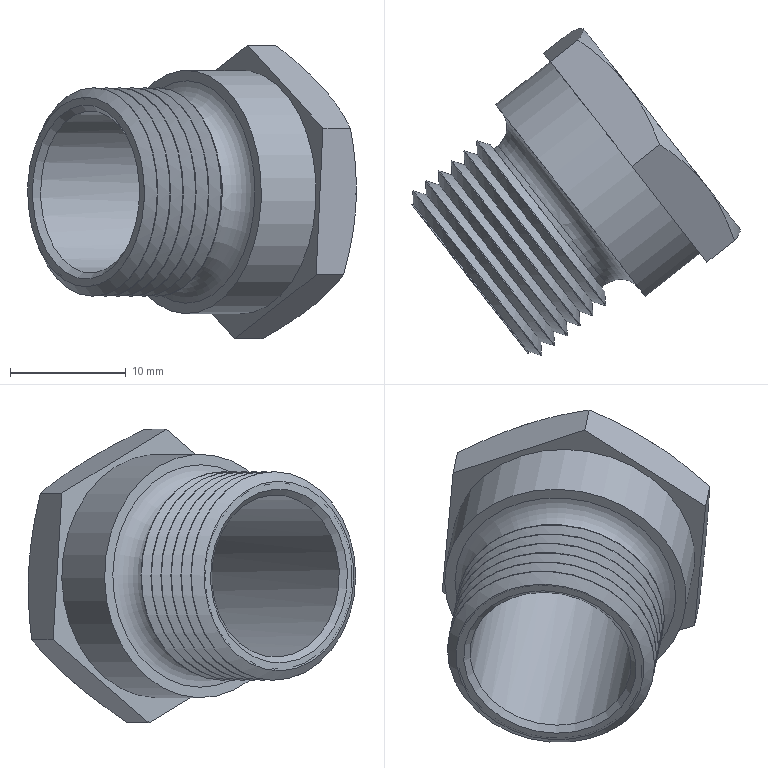Part | NX | features BREP 1 | 1 solid | 42 faces | box 28.365 x 28.243 x 25.334 mm | volume 2943 mm3 | cone 21 | plane 11 | cylinder 9 | torus 1 | commonest cylinder face diameters 18 x6 14 x1 15.2 x1 21 x1
STEP:
#1=CARTESIAN_POINT('',(-20.726,70.701,-110.314));
#2=VERTEX_POINT('',#1);
#3=CARTESIAN_POINT('',(-23.847,74.697,-117.75));
#4=DIRECTION('',(0.788,0.6157,0.));
#5=DIRECTION('',(0.3468,-0.4439,0.8262));
#6=AXIS2_PLACEMENT_3D('',#3,#4,#5);
#7=CIRCLE('',#6,9.);
#8=EDGE_CURVE('',#2,#2,#7,.T.);
#9=ORIENTED_EDGE('',*,*,#8,.T.);
#10=EDGE_LOOP('',(#9));
#11=FACE_BOUND('',#10,.T.);
#12=CARTESIAN_POINT('',(-26.925,78.726,-125.186));
#13=VERTEX_POINT('',#12);
#14=CARTESIAN_POINT('',(-23.803,74.731,-117.75));
#15=DIRECTION('',(-0.788,-0.6157,0.));
#16=DIRECTION('',(-0.3468,0.4439,-0.8262));
#17=AXIS2_PLACEMENT_3D('',#14,#15,#16);
#18=CIRCLE('',#17,9.);
#19=EDGE_CURVE('',#13,#13,#18,.T.);
#20=ORIENTED_EDGE('',*,*,#19,.T.);
#21=EDGE_LOOP('',(#20));
#22=FACE_BOUND('',#21,.T.);
#23=CARTESIAN_POINT('',(-25.559,73.359,-117.75));
#24=DIRECTION('',(0.788,0.6157,0.));
#25=DIRECTION('',(-0.3468,0.4439,-0.8262));
#26=AXIS2_PLACEMENT_3D('',#23,#24,#25);
#27=CYLINDRICAL_SURFACE('',#26,9.);
#28=ADVANCED_FACE('',(#11,#22),#27,.T.);
#29=CARTESIAN_POINT('',(-19.623,71.563,-110.314));
#30=VERTEX_POINT('',#29);
#31=CARTESIAN_POINT('',(-22.744,75.559,-117.75));
#32=DIRECTION('',(0.788,0.6157,0.));
#33=DIRECTION('',(0.3468,-0.4439,0.8262));
#34=AXIS2_PLACEMENT_3D('',#31,#32,#33);
#35=CIRCLE('',#34,9.);
#36=EDGE_CURVE('',#30,#30,#35,.T.);
#37=ORIENTED_EDGE('',*,*,#36,.T.);
#38=EDGE_LOOP('',(#37));
#39=FACE_BOUND('',#38,.T.);
#40=CARTESIAN_POINT('',(-25.822,79.588,-125.186));
#41=VERTEX_POINT('',#40);
#42=CARTESIAN_POINT('',(-22.7,75.593,-117.75));
#43=DIRECTION('',(-0.788,-0.6157,0.));
#44=DIRECTION('',(-0.3468,0.4439,-0.8262));
#45=AXIS2_PLACEMENT_3D('',#42,#43,#44);
#46=CIRCLE('',#45,9.);
#47=EDGE_CURVE('',#41,#41,#46,.T.);
#48=ORIENTED_EDGE('',*,*,#47,.T.);
#49=EDGE_LOOP('',(#48));
#50=FACE_BOUND('',#49,.T.);
#51=CARTESIAN_POINT('',(-25.559,73.359,-117.75));
#52=DIRECTION('',(0.788,0.6157,0.));
#53=DIRECTION('',(-0.3468,0.4439,-0.8262));
#54=AXIS2_PLACEMENT_3D('',#51,#52,#53);
#55=CYLINDRICAL_SURFACE('',#54,9.);
#56=ADVANCED_FACE('',(#39,#50),#55,.T.);
#57=CARTESIAN_POINT('',(-18.52,72.425,-110.314));
#58=VERTEX_POINT('',#57);
#59=CARTESIAN_POINT('',(-21.641,76.42,-117.75));
#60=DIRECTION('',(0.788,0.6157,0.));
#61=DIRECTION('',(0.3468,-0.4439,0.8262));
#62=AXIS2_PLACEMENT_3D('',#59,#60,#61);
#63=CIRCLE('',#62,9.);
#64=EDGE_CURVE('',#58,#58,#63,.T.);
#65=ORIENTED_EDGE('',*,*,#64,.T.);
#66=EDGE_LOOP('',(#65));
#67=FACE_BOUND('',#66,.T.);
#68=CARTESIAN_POINT('',(-24.718,80.45,-125.186));
#69=VERTEX_POINT('',#68);
#70=CARTESIAN_POINT('',(-21.597,76.455,-117.75));
#71=DIRECTION('',(-0.788,-0.6157,0.));
#72=DIRECTION('',(-0.3468,0.4439,-0.8262));
#73=AXIS2_PLACEMENT_3D('',#70,#71,#72);
#74=CIRCLE('',#73,9.);
#75=EDGE_CURVE('',#69,#69,#74,.T.);
#76=ORIENTED_EDGE('',*,*,#75,.T.);
#77=EDGE_LOOP('',(#76));
#78=FACE_BOUND('',#77,.T.);
#79=CARTESIAN_POINT('',(-25.559,73.359,-117.75));
#80=DIRECTION('',(0.788,0.6157,0.));
#81=DIRECTION('',(-0.3468,0.4439,-0.8262));
#82=AXIS2_PLACEMENT_3D('',#79,#80,#81);
#83=CYLINDRICAL_SURFACE('',#82,9.);
#84=ADVANCED_FACE('',(#67,#78),#83,.T.);
#85=CARTESIAN_POINT('',(-17.416,73.287,-110.314));
#86=VERTEX_POINT('',#85);
#87=CARTESIAN_POINT('',(-20.538,77.282,-117.75));
#88=DIRECTION('',(0.788,0.6157,0.));
#89=DIRECTION('',(0.3468,-0.4439,0.8262));
#90=AXIS2_PLACEMENT_3D('',#87,#88,#89);
#91=CIRCLE('',#90,9.);
#92=EDGE_CURVE('',#86,#86,#91,.T.);
#93=ORIENTED_EDGE('',*,*,#92,.T.);
#94=EDGE_LOOP('',(#93));
#95=FACE_BOUND('',#94,.T.);
#96=CARTESIAN_POINT('',(-23.615,81.312,-125.186));
#97=VERTEX_POINT('',#96);
#98=CARTESIAN_POINT('',(-20.494,77.317,-117.75));
#99=DIRECTION('',(-0.788,-0.6157,0.));
#100=DIRECTION('',(-0.3468,0.4439,-0.8262));
#101=AXIS2_PLACEMENT_3D('',#98,#99,#100);
#102=CIRCLE('',#101,9.);
#103=EDGE_CURVE('',#97,#97,#102,.T.);
#104=ORIENTED_EDGE('',*,*,#103,.T.);
#105=EDGE_LOOP('',(#104));
#106=FACE_BOUND('',#105,.T.);
#107=CARTESIAN_POINT('',(-25.559,73.359,-117.75));
#108=DIRECTION('',(0.788,0.6157,0.));
#109=DIRECTION('',(-0.3468,0.4439,-0.8262));
#110=AXIS2_PLACEMENT_3D('',#107,#108,#109);
#111=CYLINDRICAL_SURFACE('',#110,9.);
#112=ADVANCED_FACE('',(#95,#106),#111,.T.);
#113=CARTESIAN_POINT('',(-16.313,74.149,-110.314));
#114=VERTEX_POINT('',#113);
#115=CARTESIAN_POINT('',(-19.435,78.144,-117.75));
#116=DIRECTION('',(0.788,0.6157,0.));
#117=DIRECTION('',(0.3468,-0.4439,0.8262));
#118=AXIS2_PLACEMENT_3D('',#115,#116,#117);
#119=CIRCLE('',#118,9.);
#120=EDGE_CURVE('',#114,#114,#119,.T.);
#121=ORIENTED_EDGE('',*,*,#120,.T.);
#122=EDGE_LOOP('',(#121));
#123=FACE_BOUND('',#122,.T.);
#124=CARTESIAN_POINT('',(-22.512,82.174,-125.186));
#125=VERTEX_POINT('',#124);
#126=CARTESIAN_POINT('',(-19.391,78.179,-117.75));
#127=DIRECTION('',(-0.788,-0.6157,0.));
#128=DIRECTION('',(-0.3468,0.4439,-0.8262));
#129=AXIS2_PLACEMENT_3D('',#126,#127,#128);
#130=CIRCLE('',#129,9.);
#131=EDGE_CURVE('',#125,#125,#130,.T.);
#132=ORIENTED_EDGE('',*,*,#131,.T.);
#133=EDGE_LOOP('',(#132));
#134=FACE_BOUND('',#133,.T.);
#135=CARTESIAN_POINT('',(-25.559,73.359,-117.75));
#136=DIRECTION('',(0.788,0.6157,0.));
#137=DIRECTION('',(-0.3468,0.4439,-0.8262));
#138=AXIS2_PLACEMENT_3D('',#135,#136,#137);
#139=CYLINDRICAL_SURFACE('',#138,9.);
#140=ADVANCED_FACE('',(#123,#134),#139,.T.);
#141=CARTESIAN_POINT('',(-3.324,77.415,-124.905));
#142=VERTEX_POINT('',#141);
#143=CARTESIAN_POINT('',(-6.071,82.526,-127.66));
#144=VERTEX_POINT('',#143);
#145=CARTESIAN_POINT('',(-3.324,77.415,-124.905));
#146=CARTESIAN_POINT('',(-4.003,79.256,-125.805));
#147=CARTESIAN_POINT('',(-4.87,80.988,-126.719));
#148=CARTESIAN_POINT('',(-6.071,82.526,-127.66));
#149=B_SPLINE_CURVE_WITH_KNOTS('',3,(#145,#146,#147,#148),.UNSPECIFIED.,.F.,.F.,(4,4),(0.,0.006423),.UNSPECIFIED.);
#150=EDGE_CURVE('',#142,#144,#149,.T.);
#151=ORIENTED_EDGE('',*,*,#150,.F.);
#152=CARTESIAN_POINT('',(-5.703,75.557,-124.905));
#153=VERTEX_POINT('',#152);
#154=CARTESIAN_POINT('',(-5.703,75.557,-124.905));
#155=DIRECTION('',(0.788,0.6157,0.));
#156=VECTOR('',#155,1000.);
#157=LINE('',#154,#156);
#158=EDGE_CURVE('',#153,#142,#157,.T.);
#159=ORIENTED_EDGE('',*,*,#158,.F.);
#160=CARTESIAN_POINT('',(-12.747,84.573,-130.417));
#161=VERTEX_POINT('',#160);
#162=CARTESIAN_POINT('',(-12.747,84.573,-130.417));
#163=DIRECTION('',(0.5546,-0.7099,0.4341));
#164=VECTOR('',#163,1000.);
#165=LINE('',#162,#164);
#166=EDGE_CURVE('',#161,#153,#165,.T.);
#167=ORIENTED_EDGE('',*,*,#166,.F.);
#168=CARTESIAN_POINT('',(-10.369,86.43,-130.417));
#169=VERTEX_POINT('',#168);
#170=CARTESIAN_POINT('',(-12.747,84.573,-130.417));
#171=DIRECTION('',(0.788,0.6157,0.));
#172=VECTOR('',#171,1000.);
#173=LINE('',#170,#172);
#174=EDGE_CURVE('',#161,#169,#173,.T.);
#175=ORIENTED_EDGE('',*,*,#174,.T.);
#176=CARTESIAN_POINT('',(-6.071,82.526,-127.66));
#177=CARTESIAN_POINT('',(-7.274,84.065,-128.601));
#178=CARTESIAN_POINT('',(-8.746,85.326,-129.516));
#179=CARTESIAN_POINT('',(-10.369,86.43,-130.417));
#180=B_SPLINE_CURVE_WITH_KNOTS('',3,(#176,#177,#178,#179),.UNSPECIFIED.,.F.,.F.,(4,4),(0.,0.006428),.UNSPECIFIED.);
#181=EDGE_CURVE('',#144,#169,#180,.T.);
#182=ORIENTED_EDGE('',*,*,#181,.F.);
#183=EDGE_LOOP('',(#151,#159,#167,#175,#182));
#184=FACE_BOUND('',#183,.T.);
#185=CARTESIAN_POINT('',(-12.747,84.573,-130.417));
#186=DIRECTION('',(-0.2672,0.342,0.9009));
#187=DIRECTION('',(0.5546,-0.7099,0.4341));
#188=AXIS2_PLACEMENT_3D('',#185,#186,#187);
#189=PLANE('',#188);
#190=ADVANCED_FACE('',(#184),#189,.F.);
#191=CARTESIAN_POINT('',(-2.739,76.664,-112.24));
#192=VERTEX_POINT('',#191);
#193=CARTESIAN_POINT('',(-2.258,77.645,-118.575));
#194=VERTEX_POINT('',#193);
#195=CARTESIAN_POINT('',(-2.739,76.664,-112.24));
#196=CARTESIAN_POINT('',(-2.362,77.156,-114.31));
#197=CARTESIAN_POINT('',(-2.157,77.516,-116.413));
#198=CARTESIAN_POINT('',(-2.258,77.645,-118.575));
#199=B_SPLINE_CURVE_WITH_KNOTS('',3,(#195,#196,#197,#198),.UNSPECIFIED.,.F.,.F.,(4,4),(0.,0.006428),.UNSPECIFIED.);
#200=EDGE_CURVE('',#192,#194,#199,.T.);
#201=ORIENTED_EDGE('',*,*,#200,.F.);
#202=CARTESIAN_POINT('',(-5.116,74.806,-112.24));
#203=VERTEX_POINT('',#202);
#204=CARTESIAN_POINT('',(-5.116,74.806,-112.24));
#205=DIRECTION('',(0.788,0.6157,0.));
#206=VECTOR('',#205,1000.);
#207=LINE('',#204,#206);
#208=EDGE_CURVE('',#203,#192,#207,.T.);
#209=ORIENTED_EDGE('',*,*,#208,.F.);
#210=CARTESIAN_POINT('',(-5.116,74.806,-112.24));
#211=DIRECTION('',(0.04618,-0.05911,0.9972));
#212=VECTOR('',#211,1000.);
#213=LINE('',#210,#212);
#214=EDGE_CURVE('',#153,#203,#213,.T.);
#215=ORIENTED_EDGE('',*,*,#214,.F.);
#216=ORIENTED_EDGE('',*,*,#158,.T.);
#217=CARTESIAN_POINT('',(-2.258,77.645,-118.575));
#218=CARTESIAN_POINT('',(-2.358,77.773,-120.735));
#219=CARTESIAN_POINT('',(-2.757,77.661,-122.837));
#220=CARTESIAN_POINT('',(-3.324,77.415,-124.905));
#221=B_SPLINE_CURVE_WITH_KNOTS('',3,(#217,#218,#219,#220),.UNSPECIFIED.,.F.,.F.,(4,4),(0.,0.006423),.UNSPECIFIED.);
#222=EDGE_CURVE('',#194,#142,#221,.T.);
#223=ORIENTED_EDGE('',*,*,#222,.F.);
#224=EDGE_LOOP('',(#201,#209,#215,#216,#223));
#225=FACE_BOUND('',#224,.T.);
#226=CARTESIAN_POINT('',(-5.116,74.806,-112.24));
#227=DIRECTION('',(-0.6139,0.7858,0.07501));
#228=DIRECTION('',(0.04618,-0.05911,0.9972));
#229=AXIS2_PLACEMENT_3D('',#226,#227,#228);
#230=PLANE('',#229);
#231=ADVANCED_FACE('',(#225),#230,.F.);
#232=CARTESIAN_POINT('',(-9.202,84.936,-105.083));
#233=VERTEX_POINT('',#232);
#234=CARTESIAN_POINT('',(-5.196,81.405,-108.662));
#235=VERTEX_POINT('',#234);
#236=CARTESIAN_POINT('',(-9.202,84.936,-105.083));
#237=CARTESIAN_POINT('',(-7.674,83.953,-106.252));
#238=CARTESIAN_POINT('',(-6.299,82.817,-107.44));
#239=CARTESIAN_POINT('',(-5.196,81.405,-108.662));
#240=B_SPLINE_CURVE_WITH_KNOTS('',3,(#236,#237,#238,#239),.UNSPECIFIED.,.F.,.F.,(4,4),(0.,0.006428),.UNSPECIFIED.);
#241=EDGE_CURVE('',#233,#235,#240,.T.);
#242=ORIENTED_EDGE('',*,*,#241,.F.);
#243=CARTESIAN_POINT('',(-11.579,83.078,-105.083));
#244=VERTEX_POINT('',#243);
#245=CARTESIAN_POINT('',(-11.579,83.078,-105.083));
#246=DIRECTION('',(0.788,0.6157,0.));
#247=VECTOR('',#246,1000.);
#248=LINE('',#245,#247);
#249=EDGE_CURVE('',#244,#233,#248,.T.);
#250=ORIENTED_EDGE('',*,*,#249,.F.);
#251=CARTESIAN_POINT('',(-11.579,83.078,-105.083));
#252=DIRECTION('',(-0.5087,0.6511,0.5634));
#253=VECTOR('',#252,1000.);
#254=LINE('',#251,#253);
#255=EDGE_CURVE('',#203,#244,#254,.T.);
#256=ORIENTED_EDGE('',*,*,#255,.F.);
#257=ORIENTED_EDGE('',*,*,#208,.T.);
#258=CARTESIAN_POINT('',(-5.196,81.405,-108.662));
#259=CARTESIAN_POINT('',(-4.093,79.993,-109.883));
#260=CARTESIAN_POINT('',(-3.322,78.384,-111.071));
#261=CARTESIAN_POINT('',(-2.739,76.664,-112.24));
#262=B_SPLINE_CURVE_WITH_KNOTS('',3,(#258,#259,#260,#261),.UNSPECIFIED.,.F.,.F.,(4,4),(0.,0.006428),.UNSPECIFIED.);
#263=EDGE_CURVE('',#235,#192,#262,.T.);
#264=ORIENTED_EDGE('',*,*,#263,.F.);
#265=EDGE_LOOP('',(#242,#250,#256,#257,#264));
#266=FACE_BOUND('',#265,.T.);
#267=CARTESIAN_POINT('',(-11.579,83.078,-105.083));
#268=DIRECTION('',(-0.3468,0.4439,-0.8262));
#269=DIRECTION('',(-0.788,-0.6157,0.));
#270=AXIS2_PLACEMENT_3D('',#267,#268,#269);
#271=PLANE('',#270);
#272=ADVANCED_FACE('',(#266),#271,.F.);
#273=CARTESIAN_POINT('',(-16.244,93.953,-110.595));
#274=VERTEX_POINT('',#273);
#275=CARTESIAN_POINT('',(-11.95,90.051,-107.84));
#276=VERTEX_POINT('',#275);
#277=CARTESIAN_POINT('',(-16.244,93.953,-110.595));
#278=CARTESIAN_POINT('',(-14.623,92.849,-109.695));
#279=CARTESIAN_POINT('',(-13.152,91.589,-108.781));
#280=CARTESIAN_POINT('',(-11.95,90.051,-107.84));
#281=B_SPLINE_CURVE_WITH_KNOTS('',3,(#277,#278,#279,#280),.UNSPECIFIED.,.F.,.F.,(4,4),(0.,0.006423),.UNSPECIFIED.);
#282=EDGE_CURVE('',#274,#276,#281,.T.);
#283=ORIENTED_EDGE('',*,*,#282,.F.);
#284=CARTESIAN_POINT('',(-18.623,92.094,-110.595));
#285=VERTEX_POINT('',#284);
#286=CARTESIAN_POINT('',(-18.623,92.094,-110.595));
#287=DIRECTION('',(0.788,0.6157,0.));
#288=VECTOR('',#287,1000.);
#289=LINE('',#286,#288);
#290=EDGE_CURVE('',#285,#274,#289,.T.);
#291=ORIENTED_EDGE('',*,*,#290,.F.);
#292=CARTESIAN_POINT('',(-11.579,83.078,-105.083));
#293=DIRECTION('',(-0.5546,0.7099,-0.4341));
#294=VECTOR('',#293,1000.);
#295=LINE('',#292,#294);
#296=EDGE_CURVE('',#244,#285,#295,.T.);
#297=ORIENTED_EDGE('',*,*,#296,.F.);
#298=ORIENTED_EDGE('',*,*,#249,.T.);
#299=CARTESIAN_POINT('',(-11.95,90.051,-107.84));
#300=CARTESIAN_POINT('',(-10.748,88.511,-106.899));
#301=CARTESIAN_POINT('',(-9.88,86.778,-105.984));
#302=CARTESIAN_POINT('',(-9.202,84.936,-105.083));
#303=B_SPLINE_CURVE_WITH_KNOTS('',3,(#299,#300,#301,#302),.UNSPECIFIED.,.F.,.F.,(4,4),(0.,0.006428),.UNSPECIFIED.);
#304=EDGE_CURVE('',#276,#233,#303,.T.);
#305=ORIENTED_EDGE('',*,*,#304,.F.);
#306=EDGE_LOOP('',(#283,#291,#297,#298,#305));
#307=FACE_BOUND('',#306,.T.);
#308=CARTESIAN_POINT('',(-11.579,83.078,-105.083));
#309=DIRECTION('',(0.2672,-0.342,-0.9009));
#310=DIRECTION('',(-0.5546,0.7099,-0.4341));
#311=AXIS2_PLACEMENT_3D('',#308,#309,#310);
#312=PLANE('',#311);
#313=ADVANCED_FACE('',(#307),#312,.F.);
#314=CARTESIAN_POINT('',(-16.832,94.702,-123.26));
#315=VERTEX_POINT('',#314);
#316=CARTESIAN_POINT('',(-15.764,94.932,-116.925));
#317=VERTEX_POINT('',#316);
#318=CARTESIAN_POINT('',(-16.832,94.702,-123.26));
#319=CARTESIAN_POINT('',(-16.264,94.949,-121.19));
#320=CARTESIAN_POINT('',(-15.864,95.06,-119.087));
#321=CARTESIAN_POINT('',(-15.764,94.932,-116.925));
#322=B_SPLINE_CURVE_WITH_KNOTS('',3,(#318,#319,#320,#321),.UNSPECIFIED.,.F.,.F.,(4,4),(0.,0.006428),.UNSPECIFIED.);
#323=EDGE_CURVE('',#315,#317,#322,.T.);
#324=ORIENTED_EDGE('',*,*,#323,.F.);
#325=CARTESIAN_POINT('',(-19.209,92.845,-123.26));
#326=VERTEX_POINT('',#325);
#327=CARTESIAN_POINT('',(-19.209,92.845,-123.26));
#328=DIRECTION('',(0.788,0.6157,0.));
#329=VECTOR('',#328,1000.);
#330=LINE('',#327,#329);
#331=EDGE_CURVE('',#326,#315,#330,.T.);
#332=ORIENTED_EDGE('',*,*,#331,.F.);
#333=CARTESIAN_POINT('',(-19.209,92.845,-123.26));
#334=DIRECTION('',(-0.04618,0.05911,-0.9972));
#335=VECTOR('',#334,1000.);
#336=LINE('',#333,#335);
#337=EDGE_CURVE('',#285,#326,#336,.T.);
#338=ORIENTED_EDGE('',*,*,#337,.F.);
#339=ORIENTED_EDGE('',*,*,#290,.T.);
#340=CARTESIAN_POINT('',(-15.764,94.932,-116.925));
#341=CARTESIAN_POINT('',(-15.664,94.804,-114.765));
#342=CARTESIAN_POINT('',(-15.869,94.444,-112.663));
#343=CARTESIAN_POINT('',(-16.244,93.953,-110.595));
#344=B_SPLINE_CURVE_WITH_KNOTS('',3,(#340,#341,#342,#343),.UNSPECIFIED.,.F.,.F.,(4,4),(0.,0.006423),.UNSPECIFIED.);
#345=EDGE_CURVE('',#317,#274,#344,.T.);
#346=ORIENTED_EDGE('',*,*,#345,.F.);
#347=EDGE_LOOP('',(#324,#332,#338,#339,#346));
#348=FACE_BOUND('',#347,.T.);
#349=CARTESIAN_POINT('',(-19.209,92.845,-123.26));
#350=DIRECTION('',(0.6139,-0.7858,-0.07501));
#351=DIRECTION('',(-0.04618,0.05911,-0.9972));
#352=AXIS2_PLACEMENT_3D('',#349,#350,#351);
#353=PLANE('',#352);
#354=ADVANCED_FACE('',(#348),#353,.F.);
#355=CARTESIAN_POINT('',(-12.826,91.172,-126.838));
#356=VERTEX_POINT('',#355);
#357=CARTESIAN_POINT('',(-10.369,86.43,-130.417));
#358=CARTESIAN_POINT('',(-10.953,88.151,-129.248));
#359=CARTESIAN_POINT('',(-11.723,89.76,-128.06));
#360=CARTESIAN_POINT('',(-12.826,91.172,-126.838));
#361=B_SPLINE_CURVE_WITH_KNOTS('',3,(#357,#358,#359,#360),.UNSPECIFIED.,.F.,.F.,(4,4),(0.,0.006428),.UNSPECIFIED.);
#362=EDGE_CURVE('',#169,#356,#361,.T.);
#363=ORIENTED_EDGE('',*,*,#362,.F.);
#364=ORIENTED_EDGE('',*,*,#174,.F.);
#365=CARTESIAN_POINT('',(-19.209,92.845,-123.26));
#366=DIRECTION('',(0.5087,-0.6511,-0.5634));
#367=VECTOR('',#366,1000.);
#368=LINE('',#365,#367);
#369=EDGE_CURVE('',#326,#161,#368,.T.);
#370=ORIENTED_EDGE('',*,*,#369,.F.);
#371=ORIENTED_EDGE('',*,*,#331,.T.);
#372=CARTESIAN_POINT('',(-12.826,91.172,-126.838));
#373=CARTESIAN_POINT('',(-13.929,92.583,-125.617));
#374=CARTESIAN_POINT('',(-15.304,93.72,-124.429));
#375=CARTESIAN_POINT('',(-16.832,94.702,-123.26));
#376=B_SPLINE_CURVE_WITH_KNOTS('',3,(#372,#373,#374,#375),.UNSPECIFIED.,.F.,.F.,(4,4),(0.,0.006428),.UNSPECIFIED.);
#377=EDGE_CURVE('',#356,#315,#376,.T.);
#378=ORIENTED_EDGE('',*,*,#377,.F.);
#379=EDGE_LOOP('',(#363,#364,#370,#371,#378));
#380=FACE_BOUND('',#379,.T.);
#381=CARTESIAN_POINT('',(-19.209,92.845,-123.26));
#382=DIRECTION('',(0.3468,-0.4439,0.8262));
#383=DIRECTION('',(0.788,0.6157,0.));
#384=AXIS2_PLACEMENT_3D('',#381,#382,#383);
#385=PLANE('',#384);
#386=ADVANCED_FACE('',(#380),#385,.F.);
#387=ORIENTED_EDGE('',*,*,#166,.T.);
#388=ORIENTED_EDGE('',*,*,#214,.T.);
#389=ORIENTED_EDGE('',*,*,#255,.T.);
#390=ORIENTED_EDGE('',*,*,#296,.T.);
#391=ORIENTED_EDGE('',*,*,#337,.T.);
#392=ORIENTED_EDGE('',*,*,#369,.T.);
#393=EDGE_LOOP('',(#387,#388,#389,#390,#391,#392));
#394=FACE_BOUND('',#393,.T.);
#395=CARTESIAN_POINT('',(-15.805,88.487,-126.425));
#396=VERTEX_POINT('',#395);
#397=CARTESIAN_POINT('',(-12.163,83.826,-117.75));
#398=DIRECTION('',(-0.788,-0.6157,0.));
#399=DIRECTION('',(-0.3468,0.4439,-0.8262));
#400=AXIS2_PLACEMENT_3D('',#397,#398,#399);
#401=CIRCLE('',#400,10.5);
#402=EDGE_CURVE('',#396,#396,#401,.T.);
#403=ORIENTED_EDGE('',*,*,#402,.F.);
#404=EDGE_LOOP('',(#403));
#405=FACE_BOUND('',#404,.T.);
#406=CARTESIAN_POINT('',(1.341,66.541,-119.392));
#407=DIRECTION('',(0.788,0.6157,0.));
#408=DIRECTION('',(-0.3468,0.4439,-0.8262));
#409=AXIS2_PLACEMENT_3D('',#406,#407,#408);
#410=PLANE('',#409);
#411=ADVANCED_FACE('',(#394,#405),#410,.F.);
#412=CARTESIAN_POINT('',(-20.533,84.793,-126.425));
#413=VERTEX_POINT('',#412);
#414=CARTESIAN_POINT('',(-16.891,80.132,-117.75));
#415=DIRECTION('',(-0.788,-0.6157,0.));
#416=DIRECTION('',(-0.3468,0.4439,-0.8262));
#417=AXIS2_PLACEMENT_3D('',#414,#415,#416);
#418=CIRCLE('',#417,10.5);
#419=EDGE_CURVE('',#413,#413,#418,.T.);
#420=ORIENTED_EDGE('',*,*,#419,.F.);
#421=EDGE_LOOP('',(#420));
#422=FACE_BOUND('',#421,.T.);
#423=ORIENTED_EDGE('',*,*,#402,.T.);
#424=EDGE_LOOP('',(#423));
#425=FACE_BOUND('',#424,.T.);
#426=CARTESIAN_POINT('',(-16.891,80.132,-117.75));
#427=DIRECTION('',(0.788,0.6157,0.));
#428=DIRECTION('',(-0.3468,0.4439,-0.8262));
#429=AXIS2_PLACEMENT_3D('',#426,#427,#428);
#430=CYLINDRICAL_SURFACE('',#429,10.5);
#431=ADVANCED_FACE('',(#422,#425),#430,.T.);
#432=CARTESIAN_POINT('',(-20.221,84.393,-125.682));
#433=VERTEX_POINT('',#432);
#434=CARTESIAN_POINT('',(-16.891,80.132,-117.75));
#435=DIRECTION('',(0.788,0.6157,0.));
#436=DIRECTION('',(-0.3468,0.4439,-0.8262));
#437=AXIS2_PLACEMENT_3D('',#434,#435,#436);
#438=CIRCLE('',#437,9.6);
#439=EDGE_CURVE('',#433,#433,#438,.T.);
#440=ORIENTED_EDGE('',*,*,#439,.T.);
#441=EDGE_LOOP('',(#440));
#442=FACE_BOUND('',#441,.T.);
#443=ORIENTED_EDGE('',*,*,#419,.T.);
#444=EDGE_LOOP('',(#443));
#445=FACE_BOUND('',#444,.T.);
#446=CARTESIAN_POINT('',(-16.891,80.132,-117.75));
#447=DIRECTION('',(-0.788,-0.6157,0.));
#448=DIRECTION('',(0.3468,-0.4439,0.8262));
#449=AXIS2_PLACEMENT_3D('',#446,#447,#448);
#450=PLANE('',#449);
#451=ADVANCED_FACE('',(#442,#445),#450,.T.);
#452=ORIENTED_EDGE('',*,*,#263,.T.);
#453=ORIENTED_EDGE('',*,*,#200,.T.);
#454=CARTESIAN_POINT('',(-9.011,86.288,-117.75));
#455=DIRECTION('',(0.788,0.6157,0.));
#456=DIRECTION('',(0.3468,-0.4439,0.8262));
#457=AXIS2_PLACEMENT_3D('',#454,#455,#456);
#458=CIRCLE('',#457,11.);
#459=EDGE_CURVE('',#235,#194,#458,.T.);
#460=ORIENTED_EDGE('',*,*,#459,.F.);
#461=EDGE_LOOP('',(#452,#453,#460));
#462=FACE_BOUND('',#461,.T.);
#463=CARTESIAN_POINT('',(-9.011,86.288,-117.75));
#464=DIRECTION('',(-0.788,-0.6157,0.));
#465=DIRECTION('',(-0.3468,0.4439,-0.8262));
#466=AXIS2_PLACEMENT_3D('',#463,#464,#465);
#467=CONICAL_SURFACE('',#466,11.,1.047);
#468=ADVANCED_FACE('',(#462),#467,.T.);
#469=ORIENTED_EDGE('',*,*,#222,.T.);
#470=ORIENTED_EDGE('',*,*,#150,.T.);
#471=CARTESIAN_POINT('',(-9.011,86.288,-117.75));
#472=DIRECTION('',(-0.788,-0.6157,0.));
#473=DIRECTION('',(0.3468,-0.4439,0.8262));
#474=AXIS2_PLACEMENT_3D('',#471,#472,#473);
#475=CIRCLE('',#474,11.);
#476=EDGE_CURVE('',#144,#194,#475,.T.);
#477=ORIENTED_EDGE('',*,*,#476,.T.);
#478=EDGE_LOOP('',(#469,#470,#477));
#479=FACE_BOUND('',#478,.T.);
#480=CARTESIAN_POINT('',(-9.011,86.288,-117.75));
#481=DIRECTION('',(-0.788,-0.6157,0.));
#482=DIRECTION('',(-0.3468,0.4439,-0.8262));
#483=AXIS2_PLACEMENT_3D('',#480,#481,#482);
#484=CONICAL_SURFACE('',#483,11.,1.047);
#485=ADVANCED_FACE('',(#479),#484,.T.);
#486=ORIENTED_EDGE('',*,*,#181,.T.);
#487=ORIENTED_EDGE('',*,*,#362,.T.);
#488=CARTESIAN_POINT('',(-9.011,86.288,-117.75));
#489=DIRECTION('',(-0.788,-0.6157,0.));
#490=DIRECTION('',(0.3468,-0.4439,0.8262));
#491=AXIS2_PLACEMENT_3D('',#488,#489,#490);
#492=CIRCLE('',#491,11.);
#493=EDGE_CURVE('',#356,#144,#492,.T.);
#494=ORIENTED_EDGE('',*,*,#493,.T.);
#495=EDGE_LOOP('',(#486,#487,#494));
#496=FACE_BOUND('',#495,.T.);
#497=CARTESIAN_POINT('',(-9.011,86.288,-117.75));
#498=DIRECTION('',(-0.788,-0.6157,0.));
#499=DIRECTION('',(-0.3468,0.4439,-0.8262));
#500=AXIS2_PLACEMENT_3D('',#497,#498,#499);
#501=CONICAL_SURFACE('',#500,11.,1.047);
#502=ADVANCED_FACE('',(#496),#501,.T.);
#503=ORIENTED_EDGE('',*,*,#323,.T.);
#504=CARTESIAN_POINT('',(-9.011,86.288,-117.75));
#505=DIRECTION('',(-0.788,-0.6157,0.));
#506=DIRECTION('',(0.3468,-0.4439,0.8262));
#507=AXIS2_PLACEMENT_3D('',#504,#505,#506);
#508=CIRCLE('',#507,11.);
#509=EDGE_CURVE('',#317,#356,#508,.T.);
#510=ORIENTED_EDGE('',*,*,#509,.T.);
#511=ORIENTED_EDGE('',*,*,#377,.T.);
#512=EDGE_LOOP('',(#503,#510,#511));
#513=FACE_BOUND('',#512,.T.);
#514=CARTESIAN_POINT('',(-9.011,86.288,-117.75));
#515=DIRECTION('',(-0.788,-0.6157,0.));
#516=DIRECTION('',(-0.3468,0.4439,-0.8262));
#517=AXIS2_PLACEMENT_3D('',#514,#515,#516);
#518=CONICAL_SURFACE('',#517,11.,1.047);
#519=ADVANCED_FACE('',(#513),#518,.T.);
#520=ORIENTED_EDGE('',*,*,#282,.T.);
#521=CARTESIAN_POINT('',(-9.011,86.288,-117.75));
#522=DIRECTION('',(-0.788,-0.6157,0.));
#523=DIRECTION('',(0.3468,-0.4439,0.8262));
#524=AXIS2_PLACEMENT_3D('',#521,#522,#523);
#525=CIRCLE('',#524,11.);
#526=EDGE_CURVE('',#276,#317,#525,.T.);
#527=ORIENTED_EDGE('',*,*,#526,.T.);
#528=ORIENTED_EDGE('',*,*,#345,.T.);
#529=EDGE_LOOP('',(#520,#527,#528));
#530=FACE_BOUND('',#529,.T.);
#531=CARTESIAN_POINT('',(-9.011,86.288,-117.75));
#532=DIRECTION('',(-0.788,-0.6157,0.));
#533=DIRECTION('',(-0.3468,0.4439,-0.8262));
#534=AXIS2_PLACEMENT_3D('',#531,#532,#533);
#535=CONICAL_SURFACE('',#534,11.,1.047);
#536=ADVANCED_FACE('',(#530),#535,.T.);
#537=ORIENTED_EDGE('',*,*,#241,.T.);
#538=CARTESIAN_POINT('',(-9.011,86.288,-117.75));
#539=DIRECTION('',(-0.788,-0.6157,0.));
#540=DIRECTION('',(0.3468,-0.4439,0.8262));
#541=AXIS2_PLACEMENT_3D('',#538,#539,#540);
#542=CIRCLE('',#541,11.);
#543=EDGE_CURVE('',#235,#276,#542,.T.);
#544=ORIENTED_EDGE('',*,*,#543,.T.);
#545=ORIENTED_EDGE('',*,*,#304,.T.);
#546=EDGE_LOOP('',(#537,#544,#545));
#547=FACE_BOUND('',#546,.T.);
#548=CARTESIAN_POINT('',(-9.011,86.288,-117.75));
#549=DIRECTION('',(-0.788,-0.6157,0.));
#550=DIRECTION('',(-0.3468,0.4439,-0.8262));
#551=AXIS2_PLACEMENT_3D('',#548,#549,#550);
#552=CONICAL_SURFACE('',#551,11.,1.047);
#553=ADVANCED_FACE('',(#547),#552,.T.);
#554=CARTESIAN_POINT('',(-6.41,82.959,-111.553));
#555=VERTEX_POINT('',#554);
#556=CARTESIAN_POINT('',(-9.011,86.288,-117.75));
#557=DIRECTION('',(-0.788,-0.6157,0.));
#558=DIRECTION('',(0.3468,-0.4439,0.8262));
#559=AXIS2_PLACEMENT_3D('',#556,#557,#558);
#560=CIRCLE('',#559,7.5);
#561=EDGE_CURVE('',#555,#555,#560,.T.);
#562=ORIENTED_EDGE('',*,*,#561,.T.);
#563=EDGE_LOOP('',(#562));
#564=FACE_BOUND('',#563,.T.);
#565=ORIENTED_EDGE('',*,*,#543,.F.);
#566=ORIENTED_EDGE('',*,*,#459,.T.);
#567=ORIENTED_EDGE('',*,*,#476,.F.);
#568=ORIENTED_EDGE('',*,*,#493,.F.);
#569=ORIENTED_EDGE('',*,*,#509,.F.);
#570=ORIENTED_EDGE('',*,*,#526,.F.);
#571=EDGE_LOOP('',(#565,#566,#567,#568,#569,#570));
#572=FACE_BOUND('',#571,.T.);
#573=CARTESIAN_POINT('',(4.493,69.004,-119.392));
#574=DIRECTION('',(0.788,0.6157,0.));
#575=DIRECTION('',(-0.3468,0.4439,-0.8262));
#576=AXIS2_PLACEMENT_3D('',#573,#574,#575);
#577=PLANE('',#576);
#578=ADVANCED_FACE('',(#564,#572),#577,.T.);
#579=CARTESIAN_POINT('',(-21.103,82.274,-124.029));
#580=VERTEX_POINT('',#579);
#581=CARTESIAN_POINT('',(-18.467,78.9,-117.75));
#582=DIRECTION('',(-0.788,-0.6157,0.));
#583=DIRECTION('',(-0.3468,0.4439,-0.8262));
#584=AXIS2_PLACEMENT_3D('',#581,#582,#583);
#585=CIRCLE('',#584,7.6);
#586=EDGE_CURVE('',#580,#580,#585,.T.);
#587=ORIENTED_EDGE('',*,*,#586,.T.);
#588=EDGE_LOOP('',(#587));
#589=FACE_BOUND('',#588,.T.);
#590=CARTESIAN_POINT('',(-16.225,75.219,-111.471));
#591=VERTEX_POINT('',#590);
#592=CARTESIAN_POINT('',(-18.861,78.593,-117.75));
#593=DIRECTION('',(0.788,0.6157,0.));
#594=DIRECTION('',(0.3468,-0.4439,0.8262));
#595=AXIS2_PLACEMENT_3D('',#592,#593,#594);
#596=CIRCLE('',#595,7.6);
#597=EDGE_CURVE('',#591,#591,#596,.T.);
#598=ORIENTED_EDGE('',*,*,#597,.T.);
#599=EDGE_LOOP('',(#598));
#600=FACE_BOUND('',#599,.T.);
#601=CARTESIAN_POINT('',(-9.011,86.288,-117.75));
#602=DIRECTION('',(0.788,0.6157,0.));
#603=DIRECTION('',(-0.3468,0.4439,-0.8262));
#604=AXIS2_PLACEMENT_3D('',#601,#602,#603);
#605=CYLINDRICAL_SURFACE('',#604,7.6);
#606=ADVANCED_FACE('',(#589,#600),#605,.T.);
#607=CARTESIAN_POINT('',(-16.072,75.023,-111.107));
#608=VERTEX_POINT('',#607);
#609=CARTESIAN_POINT('',(-18.861,78.593,-117.75));
#610=DIRECTION('',(0.788,0.6157,0.));
#611=DIRECTION('',(0.3468,-0.4439,0.8262));
#612=AXIS2_PLACEMENT_3D('',#609,#610,#611);
#613=CIRCLE('',#612,8.04);
#614=EDGE_CURVE('',#608,#608,#613,.T.);
#615=ORIENTED_EDGE('',*,*,#614,.T.);
#616=EDGE_LOOP('',(#615));
#617=FACE_BOUND('',#616,.T.);
#618=ORIENTED_EDGE('',*,*,#597,.F.);
#619=EDGE_LOOP('',(#618));
#620=FACE_BOUND('',#619,.T.);
#621=CARTESIAN_POINT('',(-15.739,74.597,-110.314));
#622=DIRECTION('',(-0.788,-0.6157,0.));
#623=DIRECTION('',(0.3468,-0.4439,0.8262));
#624=AXIS2_PLACEMENT_3D('',#621,#622,#623);
#625=PLANE('',#624);
#626=ADVANCED_FACE('',(#617,#620),#625,.F.);
#627=CARTESIAN_POINT('',(-28.397,76.992,-124.511));
#628=VERTEX_POINT('',#627);
#629=CARTESIAN_POINT('',(-25.559,73.359,-117.75));
#630=DIRECTION('',(0.788,0.6157,0.));
#631=DIRECTION('',(-0.3468,0.4439,-0.8262));
#632=AXIS2_PLACEMENT_3D('',#629,#630,#631);
#633=CIRCLE('',#632,8.183);
#634=EDGE_CURVE('',#628,#628,#633,.T.);
#635=ORIENTED_EDGE('',*,*,#634,.F.);
#636=EDGE_LOOP('',(#635));
#637=FACE_BOUND('',#636,.T.);
#638=CARTESIAN_POINT('',(-28.16,76.689,-123.947));
#639=VERTEX_POINT('',#638);
#640=CARTESIAN_POINT('',(-25.559,73.359,-117.75));
#641=DIRECTION('',(0.788,0.6157,0.));
#642=DIRECTION('',(-0.3468,0.4439,-0.8262));
#643=AXIS2_PLACEMENT_3D('',#640,#641,#642);
#644=CIRCLE('',#643,7.5);
#645=EDGE_CURVE('',#639,#639,#644,.T.);
#646=ORIENTED_EDGE('',*,*,#645,.T.);
#647=EDGE_LOOP('',(#646));
#648=FACE_BOUND('',#647,.T.);
#649=CARTESIAN_POINT('',(-25.559,73.359,-117.75));
#650=DIRECTION('',(-0.788,-0.6157,0.));
#651=DIRECTION('',(0.3468,-0.4439,0.8262));
#652=AXIS2_PLACEMENT_3D('',#649,#650,#651);
#653=PLANE('',#652);
#654=ADVANCED_FACE('',(#637,#648),#653,.T.);
#655=CARTESIAN_POINT('',(-21.829,69.839,-110.314));
#656=VERTEX_POINT('',#655);
#657=CARTESIAN_POINT('',(-24.951,73.835,-117.75));
#658=DIRECTION('',(0.788,0.6157,0.));
#659=DIRECTION('',(0.3468,-0.4439,0.8262));
#660=AXIS2_PLACEMENT_3D('',#657,#658,#659);
#661=CIRCLE('',#660,9.);
#662=EDGE_CURVE('',#656,#656,#661,.T.);
#663=ORIENTED_EDGE('',*,*,#662,.T.);
#664=EDGE_LOOP('',(#663));
#665=FACE_BOUND('',#664,.T.);
#666=CARTESIAN_POINT('',(-28.028,77.865,-125.186));
#667=VERTEX_POINT('',#666);
#668=CARTESIAN_POINT('',(-24.907,73.869,-117.75));
#669=DIRECTION('',(-0.788,-0.6157,0.));
#670=DIRECTION('',(-0.3468,0.4439,-0.8262));
#671=AXIS2_PLACEMENT_3D('',#668,#669,#670);
#672=CIRCLE('',#671,9.);
#673=EDGE_CURVE('',#667,#667,#672,.T.);
#674=ORIENTED_EDGE('',*,*,#673,.T.);
#675=EDGE_LOOP('',(#674));
#676=FACE_BOUND('',#675,.T.);
#677=CARTESIAN_POINT('',(-25.559,73.359,-117.75));
#678=DIRECTION('',(0.788,0.6157,0.));
#679=DIRECTION('',(-0.3468,0.4439,-0.8262));
#680=AXIS2_PLACEMENT_3D('',#677,#678,#679);
#681=CYLINDRICAL_SURFACE('',#680,9.);
#682=ADVANCED_FACE('',(#665,#676),#681,.T.);
#683=ORIENTED_EDGE('',*,*,#586,.F.);
#684=EDGE_LOOP('',(#683));
#685=FACE_BOUND('',#684,.T.);
#686=ORIENTED_EDGE('',*,*,#439,.F.);
#687=EDGE_LOOP('',(#686));
#688=FACE_BOUND('',#687,.T.);
#689=CARTESIAN_POINT('',(-18.467,78.9,-117.75));
#690=DIRECTION('',(-0.788,-0.6157,0.));
#691=DIRECTION('',(0.3468,-0.4439,0.8262));
#692=AXIS2_PLACEMENT_3D('',#689,#690,#691);
#693=TOROIDAL_SURFACE('',#692,9.6,2.);
#694=ADVANCED_FACE('',(#685,#688),#693,.F.);
#695=CARTESIAN_POINT('',(-27.593,76.775,-123.533));
#696=VERTEX_POINT('',#695);
#697=CARTESIAN_POINT('',(-25.165,73.667,-117.75));
#698=DIRECTION('',(-0.788,-0.6157,0.));
#699=DIRECTION('',(-0.3468,0.4439,-0.8262));
#700=AXIS2_PLACEMENT_3D('',#697,#698,#699);
#701=CIRCLE('',#700,7.);
#702=EDGE_CURVE('',#696,#696,#701,.T.);
#703=ORIENTED_EDGE('',*,*,#702,.T.);
#704=EDGE_LOOP('',(#703));
#705=FACE_BOUND('',#704,.T.);
#706=CARTESIAN_POINT('',(-6.977,82.873,-111.967));
#707=VERTEX_POINT('',#706);
#708=CARTESIAN_POINT('',(-9.405,85.98,-117.75));
#709=DIRECTION('',(0.788,0.6157,0.));
#710=DIRECTION('',(0.3468,-0.4439,0.8262));
#711=AXIS2_PLACEMENT_3D('',#708,#709,#710);
#712=CIRCLE('',#711,7.);
#713=EDGE_CURVE('',#707,#707,#712,.T.);
#714=ORIENTED_EDGE('',*,*,#713,.T.);
#715=EDGE_LOOP('',(#714));
#716=FACE_BOUND('',#715,.T.);
#717=CARTESIAN_POINT('',(-9.011,86.288,-117.75));
#718=DIRECTION('',(-0.788,-0.6157,0.));
#719=DIRECTION('',(0.3468,-0.4439,0.8262));
#720=AXIS2_PLACEMENT_3D('',#717,#718,#719);
#721=CYLINDRICAL_SURFACE('',#720,7.);
#722=ADVANCED_FACE('',(#705,#716),#721,.F.);
#723=ORIENTED_EDGE('',*,*,#645,.F.);
#724=EDGE_LOOP('',(#723));
#725=FACE_BOUND('',#724,.T.);
#726=ORIENTED_EDGE('',*,*,#702,.F.);
#727=EDGE_LOOP('',(#726));
#728=FACE_BOUND('',#727,.T.);
#729=CARTESIAN_POINT('',(-25.165,73.667,-117.75));
#730=DIRECTION('',(-0.788,-0.6157,0.));
#731=DIRECTION('',(0.3468,-0.4439,0.8262));
#732=AXIS2_PLACEMENT_3D('',#729,#730,#731);
#733=CONICAL_SURFACE('',#732,7.,0.7854);
#734=ADVANCED_FACE('',(#725,#728),#733,.F.);
#735=ORIENTED_EDGE('',*,*,#713,.F.);
#736=EDGE_LOOP('',(#735));
#737=FACE_BOUND('',#736,.T.);
#738=ORIENTED_EDGE('',*,*,#561,.F.);
#739=EDGE_LOOP('',(#738));
#740=FACE_BOUND('',#739,.T.);
#741=CARTESIAN_POINT('',(-9.011,86.288,-117.75));
#742=DIRECTION('',(0.788,0.6157,0.));
#743=DIRECTION('',(-0.3468,0.4439,-0.8262));
#744=AXIS2_PLACEMENT_3D('',#741,#742,#743);
#745=CONICAL_SURFACE('',#744,7.5,0.7854);
#746=ADVANCED_FACE('',(#737,#740),#745,.F.);
#747=ORIENTED_EDGE('',*,*,#614,.F.);
#748=EDGE_LOOP('',(#747));
#749=FACE_BOUND('',#748,.T.);
#750=ORIENTED_EDGE('',*,*,#131,.F.);
#751=EDGE_LOOP('',(#750));
#752=FACE_BOUND('',#751,.T.);
#753=CARTESIAN_POINT('',(-19.413,78.162,-117.75));
#754=DIRECTION('',(-0.788,-0.6157,0.));
#755=DIRECTION('',(0.3468,-0.4439,0.8262));
#756=AXIS2_PLACEMENT_3D('',#753,#754,#755);
#757=CONICAL_SURFACE('',#756,9.04,0.9601);
#758=ADVANCED_FACE('',(#749,#752),#757,.T.);
#759=CARTESIAN_POINT('',(-17.176,74.161,-111.107));
#760=VERTEX_POINT('',#759);
#761=CARTESIAN_POINT('',(-19.964,77.731,-117.75));
#762=DIRECTION('',(0.788,0.6157,0.));
#763=DIRECTION('',(0.3468,-0.4439,0.8262));
#764=AXIS2_PLACEMENT_3D('',#761,#762,#763);
#765=CIRCLE('',#764,8.04);
#766=EDGE_CURVE('',#760,#760,#765,.T.);
#767=ORIENTED_EDGE('',*,*,#766,.T.);
#768=EDGE_LOOP('',(#767));
#769=FACE_BOUND('',#768,.T.);
#770=ORIENTED_EDGE('',*,*,#120,.F.);
#771=EDGE_LOOP('',(#770));
#772=FACE_BOUND('',#771,.T.);
#773=CARTESIAN_POINT('',(-19.964,77.731,-117.75));
#774=DIRECTION('',(0.788,0.6157,0.));
#775=DIRECTION('',(-0.3468,0.4439,-0.8262));
#776=AXIS2_PLACEMENT_3D('',#773,#774,#775);
#777=CONICAL_SURFACE('',#776,8.04,0.9601);
#778=ADVANCED_FACE('',(#769,#772),#777,.T.);
#779=ORIENTED_EDGE('',*,*,#766,.F.);
#780=EDGE_LOOP('',(#779));
#781=FACE_BOUND('',#780,.T.);
#782=ORIENTED_EDGE('',*,*,#103,.F.);
#783=EDGE_LOOP('',(#782));
#784=FACE_BOUND('',#783,.T.);
#785=CARTESIAN_POINT('',(-20.516,77.3,-117.75));
#786=DIRECTION('',(-0.788,-0.6157,0.));
#787=DIRECTION('',(0.3468,-0.4439,0.8262));
#788=AXIS2_PLACEMENT_3D('',#785,#786,#787);
#789=CONICAL_SURFACE('',#788,9.04,0.9601);
#790=ADVANCED_FACE('',(#781,#784),#789,.T.);
#791=CARTESIAN_POINT('',(-18.279,73.299,-111.107));
#792=VERTEX_POINT('',#791);
#793=CARTESIAN_POINT('',(-21.067,76.869,-117.75));
#794=DIRECTION('',(0.788,0.6157,0.));
#795=DIRECTION('',(0.3468,-0.4439,0.8262));
#796=AXIS2_PLACEMENT_3D('',#793,#794,#795);
#797=CIRCLE('',#796,8.04);
#798=EDGE_CURVE('',#792,#792,#797,.T.);
#799=ORIENTED_EDGE('',*,*,#798,.T.);
#800=EDGE_LOOP('',(#799));
#801=FACE_BOUND('',#800,.T.);
#802=ORIENTED_EDGE('',*,*,#92,.F.);
#803=EDGE_LOOP('',(#802));
#804=FACE_BOUND('',#803,.T.);
#805=CARTESIAN_POINT('',(-21.067,76.869,-117.75));
#806=DIRECTION('',(0.788,0.6157,0.));
#807=DIRECTION('',(-0.3468,0.4439,-0.8262));
#808=AXIS2_PLACEMENT_3D('',#805,#806,#807);
#809=CONICAL_SURFACE('',#808,8.04,0.9601);
#810=ADVANCED_FACE('',(#801,#804),#809,.T.);
#811=ORIENTED_EDGE('',*,*,#798,.F.);
#812=EDGE_LOOP('',(#811));
#813=FACE_BOUND('',#812,.T.);
#814=ORIENTED_EDGE('',*,*,#75,.F.);
#815=EDGE_LOOP('',(#814));
#816=FACE_BOUND('',#815,.T.);
#817=CARTESIAN_POINT('',(-21.619,76.438,-117.75));
#818=DIRECTION('',(-0.788,-0.6157,0.));
#819=DIRECTION('',(0.3468,-0.4439,0.8262));
#820=AXIS2_PLACEMENT_3D('',#817,#818,#819);
#821=CONICAL_SURFACE('',#820,9.04,0.9601);
#822=ADVANCED_FACE('',(#813,#816),#821,.T.);
#823=CARTESIAN_POINT('',(-19.382,72.438,-111.107));
#824=VERTEX_POINT('',#823);
#825=CARTESIAN_POINT('',(-22.171,76.007,-117.75));
#826=DIRECTION('',(0.788,0.6157,0.));
#827=DIRECTION('',(0.3468,-0.4439,0.8262));
#828=AXIS2_PLACEMENT_3D('',#825,#826,#827);
#829=CIRCLE('',#828,8.04);
#830=EDGE_CURVE('',#824,#824,#829,.T.);
#831=ORIENTED_EDGE('',*,*,#830,.T.);
#832=EDGE_LOOP('',(#831));
#833=FACE_BOUND('',#832,.T.);
#834=ORIENTED_EDGE('',*,*,#64,.F.);
#835=EDGE_LOOP('',(#834));
#836=FACE_BOUND('',#835,.T.);
#837=CARTESIAN_POINT('',(-22.171,76.007,-117.75));
#838=DIRECTION('',(0.788,0.6157,0.));
#839=DIRECTION('',(-0.3468,0.4439,-0.8262));
#840=AXIS2_PLACEMENT_3D('',#837,#838,#839);
#841=CONICAL_SURFACE('',#840,8.04,0.9601);
#842=ADVANCED_FACE('',(#833,#836),#841,.T.);
#843=ORIENTED_EDGE('',*,*,#830,.F.);
#844=EDGE_LOOP('',(#843));
#845=FACE_BOUND('',#844,.T.);
#846=ORIENTED_EDGE('',*,*,#47,.F.);
#847=EDGE_LOOP('',(#846));
#848=FACE_BOUND('',#847,.T.);
#849=CARTESIAN_POINT('',(-22.722,75.576,-117.75));
#850=DIRECTION('',(-0.788,-0.6157,0.));
#851=DIRECTION('',(0.3468,-0.4439,0.8262));
#852=AXIS2_PLACEMENT_3D('',#849,#850,#851);
#853=CONICAL_SURFACE('',#852,9.04,0.9601);
#854=ADVANCED_FACE('',(#845,#848),#853,.T.);
#855=CARTESIAN_POINT('',(-20.485,71.576,-111.107));
#856=VERTEX_POINT('',#855);
#857=CARTESIAN_POINT('',(-23.274,75.145,-117.75));
#858=DIRECTION('',(0.788,0.6157,0.));
#859=DIRECTION('',(0.3468,-0.4439,0.8262));
#860=AXIS2_PLACEMENT_3D('',#857,#858,#859);
#861=CIRCLE('',#860,8.04);
#862=EDGE_CURVE('',#856,#856,#861,.T.);
#863=ORIENTED_EDGE('',*,*,#862,.T.);
#864=EDGE_LOOP('',(#863));
#865=FACE_BOUND('',#864,.T.);
#866=ORIENTED_EDGE('',*,*,#36,.F.);
#867=EDGE_LOOP('',(#866));
#868=FACE_BOUND('',#867,.T.);
#869=CARTESIAN_POINT('',(-23.274,75.145,-117.75));
#870=DIRECTION('',(0.788,0.6157,0.));
#871=DIRECTION('',(-0.3468,0.4439,-0.8262));
#872=AXIS2_PLACEMENT_3D('',#869,#870,#871);
#873=CONICAL_SURFACE('',#872,8.04,0.9601);
#874=ADVANCED_FACE('',(#865,#868),#873,.T.);
#875=ORIENTED_EDGE('',*,*,#862,.F.);
#876=EDGE_LOOP('',(#875));
#877=FACE_BOUND('',#876,.T.);
#878=ORIENTED_EDGE('',*,*,#19,.F.);
#879=EDGE_LOOP('',(#878));
#880=FACE_BOUND('',#879,.T.);
#881=CARTESIAN_POINT('',(-23.825,74.714,-117.75));
#882=DIRECTION('',(-0.788,-0.6157,0.));
#883=DIRECTION('',(0.3468,-0.4439,0.8262));
#884=AXIS2_PLACEMENT_3D('',#881,#882,#883);
#885=CONICAL_SURFACE('',#884,9.04,0.9601);
#886=ADVANCED_FACE('',(#877,#880),#885,.T.);
#887=CARTESIAN_POINT('',(-21.588,70.714,-111.107));
#888=VERTEX_POINT('',#887);
#889=CARTESIAN_POINT('',(-24.377,74.283,-117.75));
#890=DIRECTION('',(0.788,0.6157,0.));
#891=DIRECTION('',(0.3468,-0.4439,0.8262));
#892=AXIS2_PLACEMENT_3D('',#889,#890,#891);
#893=CIRCLE('',#892,8.04);
#894=EDGE_CURVE('',#888,#888,#893,.T.);
#895=ORIENTED_EDGE('',*,*,#894,.T.);
#896=EDGE_LOOP('',(#895));
#897=FACE_BOUND('',#896,.T.);
#898=ORIENTED_EDGE('',*,*,#8,.F.);
#899=EDGE_LOOP('',(#898));
#900=FACE_BOUND('',#899,.T.);
#901=CARTESIAN_POINT('',(-24.377,74.283,-117.75));
#902=DIRECTION('',(0.788,0.6157,0.));
#903=DIRECTION('',(-0.3468,0.4439,-0.8262));
#904=AXIS2_PLACEMENT_3D('',#901,#902,#903);
#905=CONICAL_SURFACE('',#904,8.04,0.9601);
#906=ADVANCED_FACE('',(#897,#900),#905,.T.);
#907=ORIENTED_EDGE('',*,*,#894,.F.);
#908=EDGE_LOOP('',(#907));
#909=FACE_BOUND('',#908,.T.);
#910=ORIENTED_EDGE('',*,*,#673,.F.);
#911=EDGE_LOOP('',(#910));
#912=FACE_BOUND('',#911,.T.);
#913=CARTESIAN_POINT('',(-24.929,73.852,-117.75));
#914=DIRECTION('',(-0.788,-0.6157,0.));
#915=DIRECTION('',(0.3468,-0.4439,0.8262));
#916=AXIS2_PLACEMENT_3D('',#913,#914,#915);
#917=CONICAL_SURFACE('',#916,9.04,0.9601);
#918=ADVANCED_FACE('',(#909,#912),#917,.T.);
#919=CARTESIAN_POINT('',(-22.692,69.852,-111.107));
#920=VERTEX_POINT('',#919);
#921=CARTESIAN_POINT('',(-25.48,73.421,-117.75));
#922=DIRECTION('',(0.788,0.6157,0.));
#923=DIRECTION('',(0.3468,-0.4439,0.8262));
#924=AXIS2_PLACEMENT_3D('',#921,#922,#923);
#925=CIRCLE('',#924,8.04);
#926=EDGE_CURVE('',#920,#920,#925,.T.);
#927=ORIENTED_EDGE('',*,*,#926,.T.);
#928=EDGE_LOOP('',(#927));
#929=FACE_BOUND('',#928,.T.);
#930=ORIENTED_EDGE('',*,*,#662,.F.);
#931=EDGE_LOOP('',(#930));
#932=FACE_BOUND('',#931,.T.);
#933=CARTESIAN_POINT('',(-25.48,73.421,-117.75));
#934=DIRECTION('',(0.788,0.6157,0.));
#935=DIRECTION('',(-0.3468,0.4439,-0.8262));
#936=AXIS2_PLACEMENT_3D('',#933,#934,#935);
#937=CONICAL_SURFACE('',#936,8.04,0.9601);
#938=ADVANCED_FACE('',(#929,#932),#937,.T.);
#939=ORIENTED_EDGE('',*,*,#634,.T.);
#940=EDGE_LOOP('',(#939));
#941=FACE_BOUND('',#940,.T.);
#942=ORIENTED_EDGE('',*,*,#926,.F.);
#943=EDGE_LOOP('',(#942));
#944=FACE_BOUND('',#943,.T.);
#945=CARTESIAN_POINT('',(-26.032,72.99,-117.75));
#946=DIRECTION('',(-0.788,-0.6157,0.));
#947=DIRECTION('',(0.3468,-0.4439,0.8262));
#948=AXIS2_PLACEMENT_3D('',#945,#946,#947);
#949=CONICAL_SURFACE('',#948,9.04,0.9601);
#950=ADVANCED_FACE('',(#941,#944),#949,.T.);
#951=CLOSED_SHELL('',(#28,#56,#84,#112,#140,#190,#231,#272,#313,#354,#386,#411,#431,#451,#468,#485,#502,#519,#536,#553,#578,#606,#626,#654,#682,#694,#722,#734,#746,#758,#778,#790,#810,#822,#842,#854,#874,#886,#906,#918,#938,#950));
#952=MANIFOLD_SOLID_BREP('',#951);
#953=(LENGTH_UNIT()NAMED_UNIT(*)SI_UNIT(.MILLI.,.METRE.));
#954=UNCERTAINTY_MEASURE_WITH_UNIT(LENGTH_MEASURE(0.0508),#953,'','');
#955=(NAMED_UNIT(*)PLANE_ANGLE_UNIT()SI_UNIT($,.RADIAN.));
#956=(NAMED_UNIT(*)SI_UNIT($,.STERADIAN.)SOLID_ANGLE_UNIT());
#957=(GEOMETRIC_REPRESENTATION_CONTEXT(3)GLOBAL_UNCERTAINTY_ASSIGNED_CONTEXT((#954))GLOBAL_UNIT_ASSIGNED_CONTEXT((#953,#955,#956))REPRESENTATION_CONTEXT('',''));
#958=ADVANCED_BREP_SHAPE_REPRESENTATION('',(#952),#957);